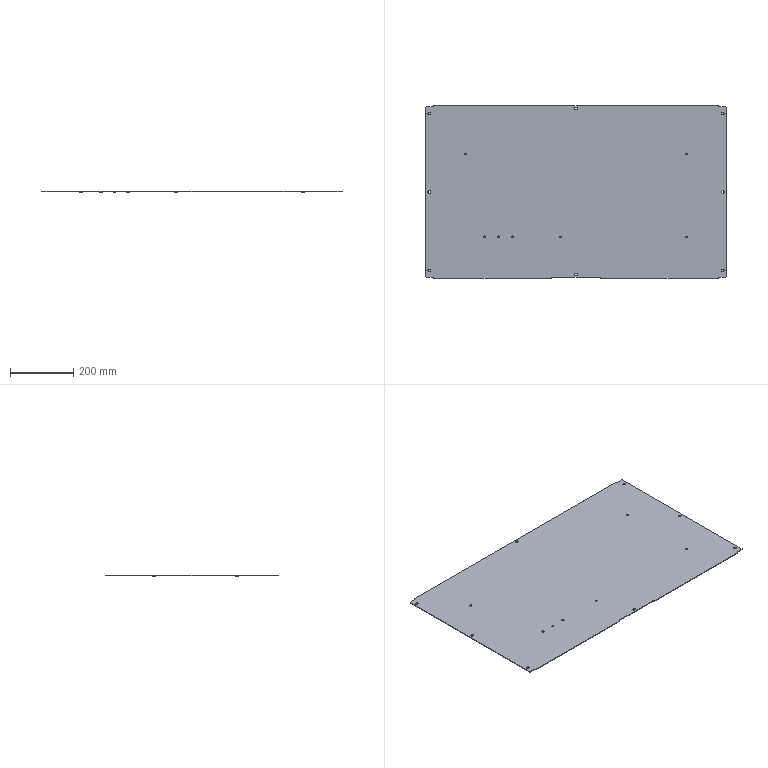Part | SolidWorks | features BaseBody 1 | 1 solid | 152 faces | box 950 x 544 x 6 mm | volume 1031940 mm3 | plane 88 | cylinder 64 | commonest cylinder face diameters 6.5 x24 5 x14 6 x12 5.5 x8 4 x6